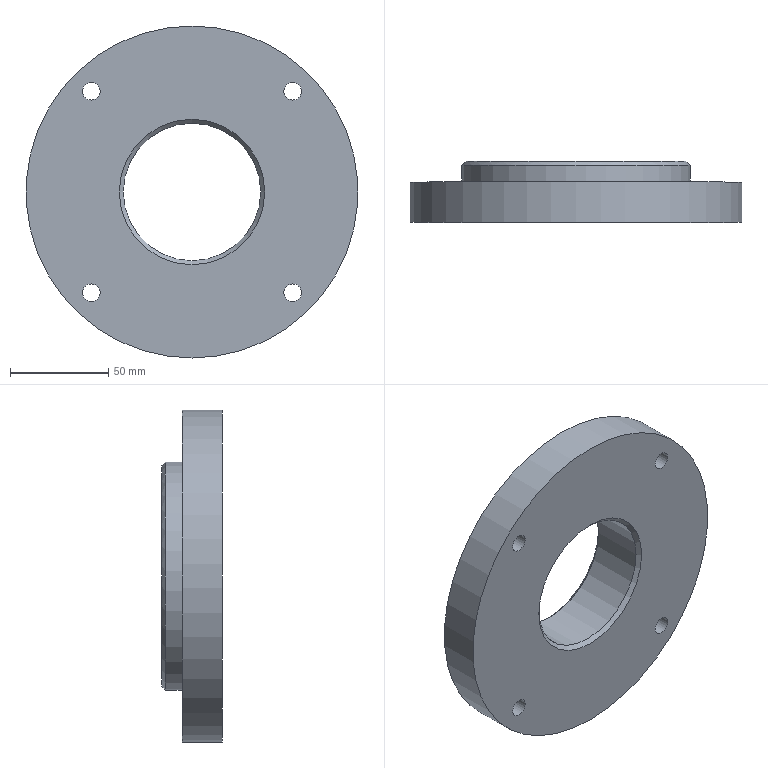Part | STEP file | LOCATING-RING_id466_x_t | 1 solid | 21 faces | box 168.974 x 31 x 168.974 mm | volume 442112 mm3 | cylinder 11 | plane 7 | cone 3 | commonest cylinder face diameters 9 x4 14 x4 70 x1 116.432 x1 168.974 x1
STEP:
#1=CARTESIAN_POINT('',(0.,191.5,-56.216));
#2=VERTEX_POINT('',#1);
#3=CARTESIAN_POINT('',(0.,191.5,0.));
#4=DIRECTION('',(0.,-1.,0.));
#5=DIRECTION('',(0.,0.,-1.));
#6=AXIS2_PLACEMENT_3D('',#3,#4,#5);
#7=CIRCLE('',#6,56.216);
#8=EDGE_CURVE('',#2,#2,#7,.T.);
#9=ORIENTED_EDGE('',*,*,#8,.T.);
#10=EDGE_LOOP('',(#9));
#11=FACE_BOUND('',#10,.T.);
#12=CARTESIAN_POINT('',(0.,189.5,-58.216));
#13=VERTEX_POINT('',#12);
#14=CARTESIAN_POINT('',(0.,189.5,0.));
#15=DIRECTION('',(0.,-1.,0.));
#16=DIRECTION('',(0.,0.,-1.));
#17=AXIS2_PLACEMENT_3D('',#14,#15,#16);
#18=CIRCLE('',#17,58.216);
#19=EDGE_CURVE('',#13,#13,#18,.T.);
#20=ORIENTED_EDGE('',*,*,#19,.F.);
#21=EDGE_LOOP('',(#20));
#22=FACE_BOUND('',#21,.T.);
#23=CARTESIAN_POINT('',(0.,189.5,0.));
#24=DIRECTION('',(0.,-1.,0.));
#25=DIRECTION('',(0.,0.,-1.));
#26=AXIS2_PLACEMENT_3D('',#23,#24,#25);
#27=CONICAL_SURFACE('',#26,58.216,45.);
#28=ADVANCED_FACE('',(#11,#22),#27,.T.);
#29=CARTESIAN_POINT('',(0.,191.5,37.));
#30=VERTEX_POINT('',#29);
#31=CARTESIAN_POINT('',(0.,191.5,0.));
#32=DIRECTION('',(0.,-1.,0.));
#33=DIRECTION('',(0.,0.,1.));
#34=AXIS2_PLACEMENT_3D('',#31,#32,#33);
#35=CIRCLE('',#34,37.);
#36=EDGE_CURVE('',#30,#30,#35,.T.);
#37=ORIENTED_EDGE('',*,*,#36,.T.);
#38=EDGE_LOOP('',(#37));
#39=FACE_BOUND('',#38,.T.);
#40=ORIENTED_EDGE('',*,*,#8,.F.);
#41=EDGE_LOOP('',(#40));
#42=FACE_BOUND('',#41,.T.);
#43=CARTESIAN_POINT('',(0.,191.5,0.));
#44=DIRECTION('',(0.,-1.,0.));
#45=DIRECTION('',(0.,0.,-1.));
#46=AXIS2_PLACEMENT_3D('',#43,#44,#45);
#47=PLANE('',#46);
#48=ADVANCED_FACE('',(#39,#42),#47,.F.);
#49=ORIENTED_EDGE('',*,*,#19,.T.);
#50=EDGE_LOOP('',(#49));
#51=FACE_BOUND('',#50,.T.);
#52=CARTESIAN_POINT('',(0.,181.,-58.216));
#53=VERTEX_POINT('',#52);
#54=CARTESIAN_POINT('',(0.,181.,0.));
#55=DIRECTION('',(0.,1.,0.));
#56=DIRECTION('',(0.,0.,-1.));
#57=AXIS2_PLACEMENT_3D('',#54,#55,#56);
#58=CIRCLE('',#57,58.216);
#59=EDGE_CURVE('',#53,#53,#58,.T.);
#60=ORIENTED_EDGE('',*,*,#59,.T.);
#61=EDGE_LOOP('',(#60));
#62=FACE_BOUND('',#61,.T.);
#63=CARTESIAN_POINT('',(0.,193.05,0.));
#64=DIRECTION('',(0.,-1.,0.));
#65=DIRECTION('',(0.,0.,-1.));
#66=AXIS2_PLACEMENT_3D('',#63,#64,#65);
#67=CYLINDRICAL_SURFACE('',#66,58.216);
#68=ADVANCED_FACE('',(#51,#62),#67,.T.);
#69=CARTESIAN_POINT('',(0.,189.5,-35.));
#70=VERTEX_POINT('',#69);
#71=CARTESIAN_POINT('',(0.,189.5,0.));
#72=DIRECTION('',(0.,-1.,0.));
#73=DIRECTION('',(0.,0.,-1.));
#74=AXIS2_PLACEMENT_3D('',#71,#72,#73);
#75=CIRCLE('',#74,35.);
#76=EDGE_CURVE('',#70,#70,#75,.T.);
#77=ORIENTED_EDGE('',*,*,#76,.T.);
#78=EDGE_LOOP('',(#77));
#79=FACE_BOUND('',#78,.T.);
#80=ORIENTED_EDGE('',*,*,#36,.F.);
#81=EDGE_LOOP('',(#80));
#82=FACE_BOUND('',#81,.T.);
#83=CARTESIAN_POINT('',(0.,191.5,0.));
#84=DIRECTION('',(0.,1.,0.));
#85=DIRECTION('',(0.,0.,1.));
#86=AXIS2_PLACEMENT_3D('',#83,#84,#85);
#87=CONICAL_SURFACE('',#86,37.,45.);
#88=ADVANCED_FACE('',(#79,#82),#87,.F.);
#89=CARTESIAN_POINT('',(51.265,172.,-44.265));
#90=VERTEX_POINT('',#89);
#91=CARTESIAN_POINT('',(51.265,172.,-51.265));
#92=DIRECTION('',(0.,1.,0.));
#93=DIRECTION('',(0.,0.,1.));
#94=AXIS2_PLACEMENT_3D('',#91,#92,#93);
#95=CIRCLE('',#94,7.);
#96=EDGE_CURVE('',#90,#90,#95,.T.);
#97=ORIENTED_EDGE('',*,*,#96,.F.);
#98=EDGE_LOOP('',(#97));
#99=FACE_BOUND('',#98,.T.);
#100=CARTESIAN_POINT('',(51.265,181.,-44.265));
#101=VERTEX_POINT('',#100);
#102=CARTESIAN_POINT('',(51.265,181.,-51.265));
#103=DIRECTION('',(0.,1.,0.));
#104=DIRECTION('',(0.,0.,1.));
#105=AXIS2_PLACEMENT_3D('',#102,#103,#104);
#106=CIRCLE('',#105,7.);
#107=EDGE_CURVE('',#101,#101,#106,.T.);
#108=ORIENTED_EDGE('',*,*,#107,.T.);
#109=EDGE_LOOP('',(#108));
#110=FACE_BOUND('',#109,.T.);
#111=CARTESIAN_POINT('',(51.265,181.,-51.265));
#112=DIRECTION('',(0.,1.,0.));
#113=DIRECTION('',(0.,0.,1.));
#114=AXIS2_PLACEMENT_3D('',#111,#112,#113);
#115=CYLINDRICAL_SURFACE('',#114,7.);
#116=ADVANCED_FACE('',(#99,#110),#115,.F.);
#117=CARTESIAN_POINT('',(51.265,172.,58.265));
#118=VERTEX_POINT('',#117);
#119=CARTESIAN_POINT('',(51.265,172.,51.265));
#120=DIRECTION('',(0.,1.,0.));
#121=DIRECTION('',(0.,0.,1.));
#122=AXIS2_PLACEMENT_3D('',#119,#120,#121);
#123=CIRCLE('',#122,7.);
#124=EDGE_CURVE('',#118,#118,#123,.T.);
#125=ORIENTED_EDGE('',*,*,#124,.F.);
#126=EDGE_LOOP('',(#125));
#127=FACE_BOUND('',#126,.T.);
#128=CARTESIAN_POINT('',(51.265,181.,58.265));
#129=VERTEX_POINT('',#128);
#130=CARTESIAN_POINT('',(51.265,181.,51.265));
#131=DIRECTION('',(0.,1.,0.));
#132=DIRECTION('',(0.,0.,1.));
#133=AXIS2_PLACEMENT_3D('',#130,#131,#132);
#134=CIRCLE('',#133,7.);
#135=EDGE_CURVE('',#129,#129,#134,.T.);
#136=ORIENTED_EDGE('',*,*,#135,.T.);
#137=EDGE_LOOP('',(#136));
#138=FACE_BOUND('',#137,.T.);
#139=CARTESIAN_POINT('',(51.265,181.,51.265));
#140=DIRECTION('',(0.,1.,0.));
#141=DIRECTION('',(0.,0.,1.));
#142=AXIS2_PLACEMENT_3D('',#139,#140,#141);
#143=CYLINDRICAL_SURFACE('',#142,7.);
#144=ADVANCED_FACE('',(#127,#138),#143,.F.);
#145=CARTESIAN_POINT('',(-51.265,172.,-44.265));
#146=VERTEX_POINT('',#145);
#147=CARTESIAN_POINT('',(-51.265,172.,-51.265));
#148=DIRECTION('',(0.,1.,0.));
#149=DIRECTION('',(0.,0.,1.));
#150=AXIS2_PLACEMENT_3D('',#147,#148,#149);
#151=CIRCLE('',#150,7.);
#152=EDGE_CURVE('',#146,#146,#151,.T.);
#153=ORIENTED_EDGE('',*,*,#152,.F.);
#154=EDGE_LOOP('',(#153));
#155=FACE_BOUND('',#154,.T.);
#156=CARTESIAN_POINT('',(-51.265,181.,-44.265));
#157=VERTEX_POINT('',#156);
#158=CARTESIAN_POINT('',(-51.265,181.,-51.265));
#159=DIRECTION('',(0.,1.,0.));
#160=DIRECTION('',(0.,0.,1.));
#161=AXIS2_PLACEMENT_3D('',#158,#159,#160);
#162=CIRCLE('',#161,7.);
#163=EDGE_CURVE('',#157,#157,#162,.T.);
#164=ORIENTED_EDGE('',*,*,#163,.T.);
#165=EDGE_LOOP('',(#164));
#166=FACE_BOUND('',#165,.T.);
#167=CARTESIAN_POINT('',(-51.265,181.,-51.265));
#168=DIRECTION('',(0.,1.,0.));
#169=DIRECTION('',(0.,0.,1.));
#170=AXIS2_PLACEMENT_3D('',#167,#168,#169);
#171=CYLINDRICAL_SURFACE('',#170,7.);
#172=ADVANCED_FACE('',(#155,#166),#171,.F.);
#173=CARTESIAN_POINT('',(-51.265,172.,58.265));
#174=VERTEX_POINT('',#173);
#175=CARTESIAN_POINT('',(-51.265,172.,51.265));
#176=DIRECTION('',(0.,1.,0.));
#177=DIRECTION('',(0.,0.,1.));
#178=AXIS2_PLACEMENT_3D('',#175,#176,#177);
#179=CIRCLE('',#178,7.);
#180=EDGE_CURVE('',#174,#174,#179,.T.);
#181=ORIENTED_EDGE('',*,*,#180,.F.);
#182=EDGE_LOOP('',(#181));
#183=FACE_BOUND('',#182,.T.);
#184=CARTESIAN_POINT('',(-51.265,181.,58.265));
#185=VERTEX_POINT('',#184);
#186=CARTESIAN_POINT('',(-51.265,181.,51.265));
#187=DIRECTION('',(0.,1.,0.));
#188=DIRECTION('',(0.,0.,1.));
#189=AXIS2_PLACEMENT_3D('',#186,#187,#188);
#190=CIRCLE('',#189,7.);
#191=EDGE_CURVE('',#185,#185,#190,.T.);
#192=ORIENTED_EDGE('',*,*,#191,.T.);
#193=EDGE_LOOP('',(#192));
#194=FACE_BOUND('',#193,.T.);
#195=CARTESIAN_POINT('',(-51.265,181.,51.265));
#196=DIRECTION('',(0.,1.,0.));
#197=DIRECTION('',(0.,0.,1.));
#198=AXIS2_PLACEMENT_3D('',#195,#196,#197);
#199=CYLINDRICAL_SURFACE('',#198,7.);
#200=ADVANCED_FACE('',(#183,#194),#199,.F.);
#201=ORIENTED_EDGE('',*,*,#135,.F.);
#202=EDGE_LOOP('',(#201));
#203=FACE_BOUND('',#202,.T.);
#204=ORIENTED_EDGE('',*,*,#191,.F.);
#205=EDGE_LOOP('',(#204));
#206=FACE_BOUND('',#205,.T.);
#207=ORIENTED_EDGE('',*,*,#163,.F.);
#208=EDGE_LOOP('',(#207));
#209=FACE_BOUND('',#208,.T.);
#210=ORIENTED_EDGE('',*,*,#107,.F.);
#211=EDGE_LOOP('',(#210));
#212=FACE_BOUND('',#211,.T.);
#213=ORIENTED_EDGE('',*,*,#59,.F.);
#214=EDGE_LOOP('',(#213));
#215=FACE_BOUND('',#214,.T.);
#216=CARTESIAN_POINT('',(0.,181.,-84.487));
#217=VERTEX_POINT('',#216);
#218=CARTESIAN_POINT('',(0.,181.,0.));
#219=DIRECTION('',(0.,-1.,0.));
#220=DIRECTION('',(0.,0.,-1.));
#221=AXIS2_PLACEMENT_3D('',#218,#219,#220);
#222=CIRCLE('',#221,84.487);
#223=EDGE_CURVE('',#217,#217,#222,.T.);
#224=ORIENTED_EDGE('',*,*,#223,.F.);
#225=EDGE_LOOP('',(#224));
#226=FACE_BOUND('',#225,.T.);
#227=CARTESIAN_POINT('',(0.,181.,0.));
#228=DIRECTION('',(0.,-1.,0.));
#229=DIRECTION('',(0.,0.,-1.));
#230=AXIS2_PLACEMENT_3D('',#227,#228,#229);
#231=PLANE('',#230);
#232=ADVANCED_FACE('',(#203,#206,#209,#212,#215,#226),#231,.F.);
#233=CARTESIAN_POINT('',(-35.,162.5,0.));
#234=VERTEX_POINT('',#233);
#235=CARTESIAN_POINT('',(0.,162.5,0.));
#236=DIRECTION('',(0.,-1.,0.));
#237=DIRECTION('',(-1.,0.,0.));
#238=AXIS2_PLACEMENT_3D('',#235,#236,#237);
#239=CIRCLE('',#238,35.);
#240=EDGE_CURVE('',#234,#234,#239,.T.);
#241=ORIENTED_EDGE('',*,*,#240,.T.);
#242=EDGE_LOOP('',(#241));
#243=FACE_BOUND('',#242,.T.);
#244=ORIENTED_EDGE('',*,*,#76,.F.);
#245=EDGE_LOOP('',(#244));
#246=FACE_BOUND('',#245,.T.);
#247=CARTESIAN_POINT('',(0.,193.05,0.));
#248=DIRECTION('',(0.,-1.,0.));
#249=DIRECTION('',(0.,0.,-1.));
#250=AXIS2_PLACEMENT_3D('',#247,#248,#249);
#251=CYLINDRICAL_SURFACE('',#250,35.);
#252=ADVANCED_FACE('',(#243,#246),#251,.F.);
#253=CARTESIAN_POINT('',(51.265,172.,-46.765));
#254=VERTEX_POINT('',#253);
#255=CARTESIAN_POINT('',(51.265,172.,-51.265));
#256=DIRECTION('',(0.,-1.,0.));
#257=DIRECTION('',(0.,0.,1.));
#258=AXIS2_PLACEMENT_3D('',#255,#256,#257);
#259=CIRCLE('',#258,4.5);
#260=EDGE_CURVE('',#254,#254,#259,.T.);
#261=ORIENTED_EDGE('',*,*,#260,.T.);
#262=EDGE_LOOP('',(#261));
#263=FACE_BOUND('',#262,.T.);
#264=ORIENTED_EDGE('',*,*,#96,.T.);
#265=EDGE_LOOP('',(#264));
#266=FACE_BOUND('',#265,.T.);
#267=CARTESIAN_POINT('',(0.,172.,0.));
#268=DIRECTION('',(0.,1.,0.));
#269=DIRECTION('',(0.,0.,1.));
#270=AXIS2_PLACEMENT_3D('',#267,#268,#269);
#271=PLANE('',#270);
#272=ADVANCED_FACE('',(#263,#266),#271,.T.);
#273=CARTESIAN_POINT('',(51.265,172.,55.765));
#274=VERTEX_POINT('',#273);
#275=CARTESIAN_POINT('',(51.265,172.,51.265));
#276=DIRECTION('',(0.,-1.,0.));
#277=DIRECTION('',(0.,0.,1.));
#278=AXIS2_PLACEMENT_3D('',#275,#276,#277);
#279=CIRCLE('',#278,4.5);
#280=EDGE_CURVE('',#274,#274,#279,.T.);
#281=ORIENTED_EDGE('',*,*,#280,.T.);
#282=EDGE_LOOP('',(#281));
#283=FACE_BOUND('',#282,.T.);
#284=ORIENTED_EDGE('',*,*,#124,.T.);
#285=EDGE_LOOP('',(#284));
#286=FACE_BOUND('',#285,.T.);
#287=CARTESIAN_POINT('',(0.,172.,0.));
#288=DIRECTION('',(0.,1.,0.));
#289=DIRECTION('',(0.,0.,1.));
#290=AXIS2_PLACEMENT_3D('',#287,#288,#289);
#291=PLANE('',#290);
#292=ADVANCED_FACE('',(#283,#286),#291,.T.);
#293=CARTESIAN_POINT('',(-51.265,172.,-46.765));
#294=VERTEX_POINT('',#293);
#295=CARTESIAN_POINT('',(-51.265,172.,-51.265));
#296=DIRECTION('',(0.,-1.,0.));
#297=DIRECTION('',(0.,0.,1.));
#298=AXIS2_PLACEMENT_3D('',#295,#296,#297);
#299=CIRCLE('',#298,4.5);
#300=EDGE_CURVE('',#294,#294,#299,.T.);
#301=ORIENTED_EDGE('',*,*,#300,.T.);
#302=EDGE_LOOP('',(#301));
#303=FACE_BOUND('',#302,.T.);
#304=ORIENTED_EDGE('',*,*,#152,.T.);
#305=EDGE_LOOP('',(#304));
#306=FACE_BOUND('',#305,.T.);
#307=CARTESIAN_POINT('',(0.,172.,0.));
#308=DIRECTION('',(0.,1.,0.));
#309=DIRECTION('',(0.,0.,1.));
#310=AXIS2_PLACEMENT_3D('',#307,#308,#309);
#311=PLANE('',#310);
#312=ADVANCED_FACE('',(#303,#306),#311,.T.);
#313=CARTESIAN_POINT('',(-51.265,172.,55.765));
#314=VERTEX_POINT('',#313);
#315=CARTESIAN_POINT('',(-51.265,172.,51.265));
#316=DIRECTION('',(0.,-1.,0.));
#317=DIRECTION('',(0.,0.,1.));
#318=AXIS2_PLACEMENT_3D('',#315,#316,#317);
#319=CIRCLE('',#318,4.5);
#320=EDGE_CURVE('',#314,#314,#319,.T.);
#321=ORIENTED_EDGE('',*,*,#320,.T.);
#322=EDGE_LOOP('',(#321));
#323=FACE_BOUND('',#322,.T.);
#324=ORIENTED_EDGE('',*,*,#180,.T.);
#325=EDGE_LOOP('',(#324));
#326=FACE_BOUND('',#325,.T.);
#327=CARTESIAN_POINT('',(0.,172.,0.));
#328=DIRECTION('',(0.,1.,0.));
#329=DIRECTION('',(0.,0.,1.));
#330=AXIS2_PLACEMENT_3D('',#327,#328,#329);
#331=PLANE('',#330);
#332=ADVANCED_FACE('',(#323,#326),#331,.T.);
#333=CARTESIAN_POINT('',(0.,160.5,-84.487));
#334=VERTEX_POINT('',#333);
#335=CARTESIAN_POINT('',(0.,160.5,0.));
#336=DIRECTION('',(0.,-1.,0.));
#337=DIRECTION('',(0.,0.,-1.));
#338=AXIS2_PLACEMENT_3D('',#335,#336,#337);
#339=CIRCLE('',#338,84.487);
#340=EDGE_CURVE('',#334,#334,#339,.T.);
#341=ORIENTED_EDGE('',*,*,#340,.F.);
#342=EDGE_LOOP('',(#341));
#343=FACE_BOUND('',#342,.T.);
#344=ORIENTED_EDGE('',*,*,#223,.T.);
#345=EDGE_LOOP('',(#344));
#346=FACE_BOUND('',#345,.T.);
#347=CARTESIAN_POINT('',(0.,193.05,0.));
#348=DIRECTION('',(0.,-1.,0.));
#349=DIRECTION('',(0.,0.,-1.));
#350=AXIS2_PLACEMENT_3D('',#347,#348,#349);
#351=CYLINDRICAL_SURFACE('',#350,84.487);
#352=ADVANCED_FACE('',(#343,#346),#351,.T.);
#353=CARTESIAN_POINT('',(0.,160.5,-37.));
#354=VERTEX_POINT('',#353);
#355=CARTESIAN_POINT('',(0.,160.5,0.));
#356=DIRECTION('',(0.,1.,0.));
#357=DIRECTION('',(0.,0.,-1.));
#358=AXIS2_PLACEMENT_3D('',#355,#356,#357);
#359=CIRCLE('',#358,37.);
#360=EDGE_CURVE('',#354,#354,#359,.T.);
#361=ORIENTED_EDGE('',*,*,#360,.F.);
#362=EDGE_LOOP('',(#361));
#363=FACE_BOUND('',#362,.T.);
#364=ORIENTED_EDGE('',*,*,#240,.F.);
#365=EDGE_LOOP('',(#364));
#366=FACE_BOUND('',#365,.T.);
#367=CARTESIAN_POINT('',(0.,160.5,0.));
#368=DIRECTION('',(0.,-1.,0.));
#369=DIRECTION('',(0.,0.,-1.));
#370=AXIS2_PLACEMENT_3D('',#367,#368,#369);
#371=CONICAL_SURFACE('',#370,37.,45.);
#372=ADVANCED_FACE('',(#363,#366),#371,.F.);
#373=CARTESIAN_POINT('',(51.265,160.5,-46.765));
#374=VERTEX_POINT('',#373);
#375=CARTESIAN_POINT('',(51.265,160.5,-51.265));
#376=DIRECTION('',(0.,1.,0.));
#377=DIRECTION('',(0.,0.,1.));
#378=AXIS2_PLACEMENT_3D('',#375,#376,#377);
#379=CIRCLE('',#378,4.5);
#380=EDGE_CURVE('',#374,#374,#379,.T.);
#381=ORIENTED_EDGE('',*,*,#380,.F.);
#382=EDGE_LOOP('',(#381));
#383=FACE_BOUND('',#382,.T.);
#384=ORIENTED_EDGE('',*,*,#260,.F.);
#385=EDGE_LOOP('',(#384));
#386=FACE_BOUND('',#385,.T.);
#387=CARTESIAN_POINT('',(51.265,181.,-51.265));
#388=DIRECTION('',(0.,1.,0.));
#389=DIRECTION('',(0.,0.,1.));
#390=AXIS2_PLACEMENT_3D('',#387,#388,#389);
#391=CYLINDRICAL_SURFACE('',#390,4.5);
#392=ADVANCED_FACE('',(#383,#386),#391,.F.);
#393=CARTESIAN_POINT('',(51.265,160.5,55.765));
#394=VERTEX_POINT('',#393);
#395=CARTESIAN_POINT('',(51.265,160.5,51.265));
#396=DIRECTION('',(0.,1.,0.));
#397=DIRECTION('',(0.,0.,1.));
#398=AXIS2_PLACEMENT_3D('',#395,#396,#397);
#399=CIRCLE('',#398,4.5);
#400=EDGE_CURVE('',#394,#394,#399,.T.);
#401=ORIENTED_EDGE('',*,*,#400,.F.);
#402=EDGE_LOOP('',(#401));
#403=FACE_BOUND('',#402,.T.);
#404=ORIENTED_EDGE('',*,*,#280,.F.);
#405=EDGE_LOOP('',(#404));
#406=FACE_BOUND('',#405,.T.);
#407=CARTESIAN_POINT('',(51.265,181.,51.265));
#408=DIRECTION('',(0.,1.,0.));
#409=DIRECTION('',(0.,0.,1.));
#410=AXIS2_PLACEMENT_3D('',#407,#408,#409);
#411=CYLINDRICAL_SURFACE('',#410,4.5);
#412=ADVANCED_FACE('',(#403,#406),#411,.F.);
#413=CARTESIAN_POINT('',(-51.265,160.5,-46.765));
#414=VERTEX_POINT('',#413);
#415=CARTESIAN_POINT('',(-51.265,160.5,-51.265));
#416=DIRECTION('',(0.,1.,0.));
#417=DIRECTION('',(0.,0.,1.));
#418=AXIS2_PLACEMENT_3D('',#415,#416,#417);
#419=CIRCLE('',#418,4.5);
#420=EDGE_CURVE('',#414,#414,#419,.T.);
#421=ORIENTED_EDGE('',*,*,#420,.F.);
#422=EDGE_LOOP('',(#421));
#423=FACE_BOUND('',#422,.T.);
#424=ORIENTED_EDGE('',*,*,#300,.F.);
#425=EDGE_LOOP('',(#424));
#426=FACE_BOUND('',#425,.T.);
#427=CARTESIAN_POINT('',(-51.265,181.,-51.265));
#428=DIRECTION('',(0.,1.,0.));
#429=DIRECTION('',(0.,0.,1.));
#430=AXIS2_PLACEMENT_3D('',#427,#428,#429);
#431=CYLINDRICAL_SURFACE('',#430,4.5);
#432=ADVANCED_FACE('',(#423,#426),#431,.F.);
#433=CARTESIAN_POINT('',(-51.265,160.5,55.765));
#434=VERTEX_POINT('',#433);
#435=CARTESIAN_POINT('',(-51.265,160.5,51.265));
#436=DIRECTION('',(0.,1.,0.));
#437=DIRECTION('',(0.,0.,1.));
#438=AXIS2_PLACEMENT_3D('',#435,#436,#437);
#439=CIRCLE('',#438,4.5);
#440=EDGE_CURVE('',#434,#434,#439,.T.);
#441=ORIENTED_EDGE('',*,*,#440,.F.);
#442=EDGE_LOOP('',(#441));
#443=FACE_BOUND('',#442,.T.);
#444=ORIENTED_EDGE('',*,*,#320,.F.);
#445=EDGE_LOOP('',(#444));
#446=FACE_BOUND('',#445,.T.);
#447=CARTESIAN_POINT('',(-51.265,181.,51.265));
#448=DIRECTION('',(0.,1.,0.));
#449=DIRECTION('',(0.,0.,1.));
#450=AXIS2_PLACEMENT_3D('',#447,#448,#449);
#451=CYLINDRICAL_SURFACE('',#450,4.5);
#452=ADVANCED_FACE('',(#443,#446),#451,.F.);
#453=ORIENTED_EDGE('',*,*,#440,.T.);
#454=EDGE_LOOP('',(#453));
#455=FACE_BOUND('',#454,.T.);
#456=ORIENTED_EDGE('',*,*,#420,.T.);
#457=EDGE_LOOP('',(#456));
#458=FACE_BOUND('',#457,.T.);
#459=ORIENTED_EDGE('',*,*,#400,.T.);
#460=EDGE_LOOP('',(#459));
#461=FACE_BOUND('',#460,.T.);
#462=ORIENTED_EDGE('',*,*,#380,.T.);
#463=EDGE_LOOP('',(#462));
#464=FACE_BOUND('',#463,.T.);
#465=ORIENTED_EDGE('',*,*,#360,.T.);
#466=EDGE_LOOP('',(#465));
#467=FACE_BOUND('',#466,.T.);
#468=ORIENTED_EDGE('',*,*,#340,.T.);
#469=EDGE_LOOP('',(#468));
#470=FACE_BOUND('',#469,.T.);
#471=CARTESIAN_POINT('',(0.,160.5,0.));
#472=DIRECTION('',(0.,-1.,0.));
#473=DIRECTION('',(0.,0.,-1.));
#474=AXIS2_PLACEMENT_3D('',#471,#472,#473);
#475=PLANE('',#474);
#476=ADVANCED_FACE('',(#455,#458,#461,#464,#467,#470),#475,.T.);
#477=CLOSED_SHELL('',(#28,#48,#68,#88,#116,#144,#172,#200,#232,#252,#272,#292,#312,#332,#352,#372,#392,#412,#432,#452,#476));
#478=MANIFOLD_SOLID_BREP('',#477);
#479=(LENGTH_UNIT()NAMED_UNIT(*)SI_UNIT(.MILLI.,.METRE.));
#480=UNCERTAINTY_MEASURE_WITH_UNIT(LENGTH_MEASURE(0.00002),#479,'','');
#481=(NAMED_UNIT(*)PLANE_ANGLE_UNIT()SI_UNIT($,.RADIAN.));
#482=PLANE_ANGLE_MEASURE_WITH_UNIT(PLANE_ANGLE_MEASURE(0.01745),#481);
#483=DIMENSIONAL_EXPONENTS(0.,0.,0.,0.,0.,0.,0.);
#484=(CONVERSION_BASED_UNIT('DEGREE',#482)NAMED_UNIT(#483)PLANE_ANGLE_UNIT());
#485=(NAMED_UNIT(*)SI_UNIT($,.STERADIAN.)SOLID_ANGLE_UNIT());
#486=(GEOMETRIC_REPRESENTATION_CONTEXT(3)GLOBAL_UNCERTAINTY_ASSIGNED_CONTEXT((#480))GLOBAL_UNIT_ASSIGNED_CONTEXT((#479,#484,#485))REPRESENTATION_CONTEXT('',''));
#487=ADVANCED_BREP_SHAPE_REPRESENTATION('',(#478),#486);